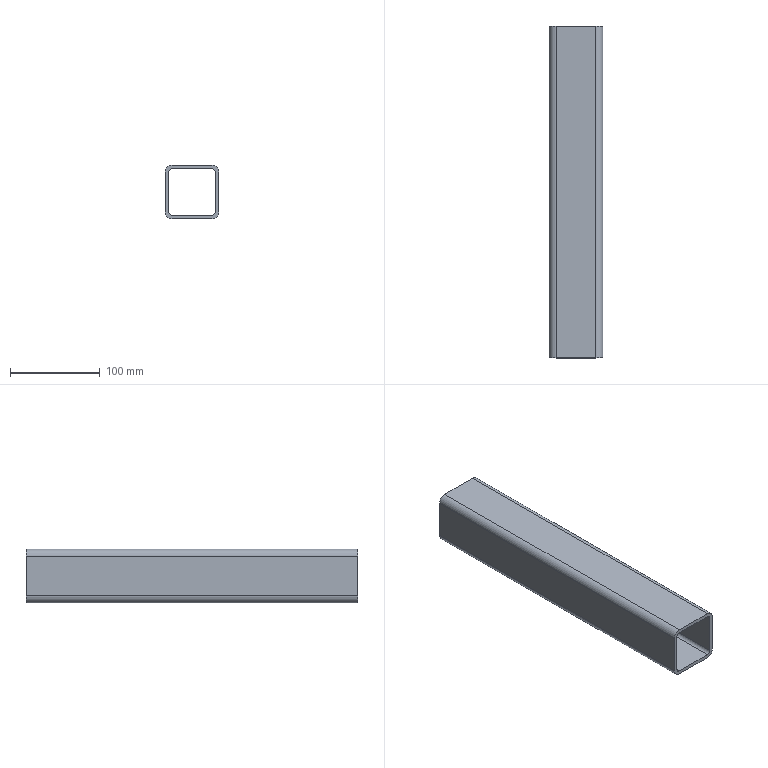Part | SolidWorks | features BaseBody 1 | 1 solid | 18 faces | box 60 x 370 x 60 mm | volume 316275 mm3 | plane 10 | cylinder 8 | commonest cylinder face diameters 8 x4 16 x4
STEP:
#1=CARTESIAN_POINT('',(26.,2432.,-1308.));
#2=VERTEX_POINT('',#1);
#3=CARTESIAN_POINT('',(26.,2432.,-1352.));
#4=VERTEX_POINT('',#3);
#5=CARTESIAN_POINT('',(26.,2432.,-1308.));
#6=DIRECTION('',(0.,0.,-1.));
#7=VECTOR('',#6,1000.);
#8=LINE('',#5,#7);
#9=EDGE_CURVE('',#2,#4,#8,.T.);
#10=ORIENTED_EDGE('',*,*,#9,.T.);
#11=CARTESIAN_POINT('',(26.,2062.,-1352.));
#12=VERTEX_POINT('',#11);
#13=CARTESIAN_POINT('',(26.,2432.,-1352.));
#14=DIRECTION('',(0.,-1.,0.));
#15=VECTOR('',#14,1000.);
#16=LINE('',#13,#15);
#17=EDGE_CURVE('',#4,#12,#16,.T.);
#18=ORIENTED_EDGE('',*,*,#17,.T.);
#19=CARTESIAN_POINT('',(26.,2062.,-1308.));
#20=VERTEX_POINT('',#19);
#21=CARTESIAN_POINT('',(26.,2062.,-1308.));
#22=DIRECTION('',(0.,0.,1.));
#23=VECTOR('',#22,1000.);
#24=LINE('',#21,#23);
#25=EDGE_CURVE('',#12,#20,#24,.T.);
#26=ORIENTED_EDGE('',*,*,#25,.T.);
#27=CARTESIAN_POINT('',(26.,2432.,-1308.));
#28=DIRECTION('',(0.,1.,0.));
#29=VECTOR('',#28,1000.);
#30=LINE('',#27,#29);
#31=EDGE_CURVE('',#20,#2,#30,.T.);
#32=ORIENTED_EDGE('',*,*,#31,.T.);
#33=EDGE_LOOP('',(#10,#18,#26,#32));
#34=FACE_OUTER_BOUND('',#33,.T.);
#35=CARTESIAN_POINT('',(26.,2432.,-1308.));
#36=DIRECTION('',(-1.,0.,0.));
#37=DIRECTION('',(0.,0.,1.));
#38=AXIS2_PLACEMENT_3D('',#35,#36,#37);
#39=PLANE('',#38);
#40=ADVANCED_FACE('',(#34),#39,.T.);
#41=ORIENTED_EDGE('',*,*,#17,.F.);
#42=CARTESIAN_POINT('',(22.,2432.,-1356.));
#43=VERTEX_POINT('',#42);
#44=CARTESIAN_POINT('',(22.,2432.,-1352.));
#45=DIRECTION('',(0.,-1.,0.));
#46=DIRECTION('',(0.,0.,-1.));
#47=AXIS2_PLACEMENT_3D('',#44,#45,#46);
#48=CIRCLE('',#47,4.);
#49=EDGE_CURVE('',#43,#4,#48,.T.);
#50=ORIENTED_EDGE('',*,*,#49,.F.);
#51=CARTESIAN_POINT('',(22.,2062.,-1356.));
#52=VERTEX_POINT('',#51);
#53=CARTESIAN_POINT('',(22.,2432.,-1356.));
#54=DIRECTION('',(0.,1.,0.));
#55=VECTOR('',#54,1000.);
#56=LINE('',#53,#55);
#57=EDGE_CURVE('',#52,#43,#56,.T.);
#58=ORIENTED_EDGE('',*,*,#57,.F.);
#59=CARTESIAN_POINT('',(22.,2062.,-1352.));
#60=DIRECTION('',(0.,1.,0.));
#61=DIRECTION('',(0.,0.,-1.));
#62=AXIS2_PLACEMENT_3D('',#59,#60,#61);
#63=CIRCLE('',#62,4.);
#64=EDGE_CURVE('',#12,#52,#63,.T.);
#65=ORIENTED_EDGE('',*,*,#64,.F.);
#66=EDGE_LOOP('',(#41,#50,#58,#65));
#67=FACE_OUTER_BOUND('',#66,.T.);
#68=CARTESIAN_POINT('',(22.,2432.,-1352.));
#69=DIRECTION('',(0.,-1.,0.));
#70=DIRECTION('',(0.,0.,-1.));
#71=AXIS2_PLACEMENT_3D('',#68,#69,#70);
#72=CYLINDRICAL_SURFACE('',#71,4.);
#73=ADVANCED_FACE('',(#67),#72,.F.);
#74=CARTESIAN_POINT('',(22.,2432.,-1304.));
#75=VERTEX_POINT('',#74);
#76=CARTESIAN_POINT('',(-22.,2432.,-1304.));
#77=VERTEX_POINT('',#76);
#78=CARTESIAN_POINT('',(-22.,2432.,-1304.));
#79=DIRECTION('',(-1.,0.,0.));
#80=VECTOR('',#79,1000.);
#81=LINE('',#78,#80);
#82=EDGE_CURVE('',#75,#77,#81,.T.);
#83=ORIENTED_EDGE('',*,*,#82,.T.);
#84=CARTESIAN_POINT('',(-26.,2432.,-1308.));
#85=VERTEX_POINT('',#84);
#86=CARTESIAN_POINT('',(-22.,2432.,-1308.));
#87=DIRECTION('',(0.,-1.,0.));
#88=DIRECTION('',(0.,0.,-1.));
#89=AXIS2_PLACEMENT_3D('',#86,#87,#88);
#90=CIRCLE('',#89,4.);
#91=EDGE_CURVE('',#77,#85,#90,.T.);
#92=ORIENTED_EDGE('',*,*,#91,.T.);
#93=CARTESIAN_POINT('',(-26.,2432.,-1352.));
#94=VERTEX_POINT('',#93);
#95=CARTESIAN_POINT('',(-26.,2432.,-1352.));
#96=DIRECTION('',(0.,0.,-1.));
#97=VECTOR('',#96,1000.);
#98=LINE('',#95,#97);
#99=EDGE_CURVE('',#85,#94,#98,.T.);
#100=ORIENTED_EDGE('',*,*,#99,.T.);
#101=CARTESIAN_POINT('',(-22.,2432.,-1356.));
#102=VERTEX_POINT('',#101);
#103=CARTESIAN_POINT('',(-22.,2432.,-1352.));
#104=DIRECTION('',(0.,-1.,0.));
#105=DIRECTION('',(0.,0.,-1.));
#106=AXIS2_PLACEMENT_3D('',#103,#104,#105);
#107=CIRCLE('',#106,4.);
#108=EDGE_CURVE('',#94,#102,#107,.T.);
#109=ORIENTED_EDGE('',*,*,#108,.T.);
#110=CARTESIAN_POINT('',(-22.,2432.,-1356.));
#111=DIRECTION('',(1.,0.,0.));
#112=VECTOR('',#111,1000.);
#113=LINE('',#110,#112);
#114=EDGE_CURVE('',#102,#43,#113,.T.);
#115=ORIENTED_EDGE('',*,*,#114,.T.);
#116=ORIENTED_EDGE('',*,*,#49,.T.);
#117=ORIENTED_EDGE('',*,*,#9,.F.);
#118=CARTESIAN_POINT('',(22.,2432.,-1308.));
#119=DIRECTION('',(0.,-1.,0.));
#120=DIRECTION('',(0.,0.,-1.));
#121=AXIS2_PLACEMENT_3D('',#118,#119,#120);
#122=CIRCLE('',#121,4.);
#123=EDGE_CURVE('',#2,#75,#122,.T.);
#124=ORIENTED_EDGE('',*,*,#123,.T.);
#125=EDGE_LOOP('',(#83,#92,#100,#109,#115,#116,#117,#124));
#126=FACE_BOUND('',#125,.T.);
#127=CARTESIAN_POINT('',(22.,2432.,-1360.));
#128=VERTEX_POINT('',#127);
#129=CARTESIAN_POINT('',(-22.,2432.,-1360.));
#130=VERTEX_POINT('',#129);
#131=CARTESIAN_POINT('',(-22.,2432.,-1360.));
#132=DIRECTION('',(-1.,0.,0.));
#133=VECTOR('',#132,1000.);
#134=LINE('',#131,#133);
#135=EDGE_CURVE('',#128,#130,#134,.T.);
#136=ORIENTED_EDGE('',*,*,#135,.T.);
#137=CARTESIAN_POINT('',(-30.,2432.,-1352.));
#138=VERTEX_POINT('',#137);
#139=CARTESIAN_POINT('',(-22.,2432.,-1352.));
#140=DIRECTION('',(0.,1.,0.));
#141=DIRECTION('',(0.,0.,-1.));
#142=AXIS2_PLACEMENT_3D('',#139,#140,#141);
#143=CIRCLE('',#142,8.);
#144=EDGE_CURVE('',#130,#138,#143,.T.);
#145=ORIENTED_EDGE('',*,*,#144,.T.);
#146=CARTESIAN_POINT('',(-30.,2432.,-1308.));
#147=VERTEX_POINT('',#146);
#148=CARTESIAN_POINT('',(-30.,2432.,-1352.));
#149=DIRECTION('',(0.,0.,1.));
#150=VECTOR('',#149,1000.);
#151=LINE('',#148,#150);
#152=EDGE_CURVE('',#138,#147,#151,.T.);
#153=ORIENTED_EDGE('',*,*,#152,.T.);
#154=CARTESIAN_POINT('',(-22.,2432.,-1300.));
#155=VERTEX_POINT('',#154);
#156=CARTESIAN_POINT('',(-22.,2432.,-1308.));
#157=DIRECTION('',(0.,1.,0.));
#158=DIRECTION('',(0.,0.,-1.));
#159=AXIS2_PLACEMENT_3D('',#156,#157,#158);
#160=CIRCLE('',#159,8.);
#161=EDGE_CURVE('',#147,#155,#160,.T.);
#162=ORIENTED_EDGE('',*,*,#161,.T.);
#163=CARTESIAN_POINT('',(22.,2432.,-1300.));
#164=VERTEX_POINT('',#163);
#165=CARTESIAN_POINT('',(-22.,2432.,-1300.));
#166=DIRECTION('',(1.,0.,0.));
#167=VECTOR('',#166,1000.);
#168=LINE('',#165,#167);
#169=EDGE_CURVE('',#155,#164,#168,.T.);
#170=ORIENTED_EDGE('',*,*,#169,.T.);
#171=CARTESIAN_POINT('',(30.,2432.,-1308.));
#172=VERTEX_POINT('',#171);
#173=CARTESIAN_POINT('',(22.,2432.,-1308.));
#174=DIRECTION('',(0.,1.,0.));
#175=DIRECTION('',(0.,0.,-1.));
#176=AXIS2_PLACEMENT_3D('',#173,#174,#175);
#177=CIRCLE('',#176,8.);
#178=EDGE_CURVE('',#164,#172,#177,.T.);
#179=ORIENTED_EDGE('',*,*,#178,.T.);
#180=CARTESIAN_POINT('',(30.,2432.,-1352.));
#181=VERTEX_POINT('',#180);
#182=CARTESIAN_POINT('',(30.,2432.,-1352.));
#183=DIRECTION('',(0.,0.,-1.));
#184=VECTOR('',#183,1000.);
#185=LINE('',#182,#184);
#186=EDGE_CURVE('',#172,#181,#185,.T.);
#187=ORIENTED_EDGE('',*,*,#186,.T.);
#188=CARTESIAN_POINT('',(22.,2432.,-1352.));
#189=DIRECTION('',(0.,1.,0.));
#190=DIRECTION('',(0.,0.,-1.));
#191=AXIS2_PLACEMENT_3D('',#188,#189,#190);
#192=CIRCLE('',#191,8.);
#193=EDGE_CURVE('',#181,#128,#192,.T.);
#194=ORIENTED_EDGE('',*,*,#193,.T.);
#195=EDGE_LOOP('',(#136,#145,#153,#162,#170,#179,#187,#194));
#196=FACE_OUTER_BOUND('',#195,.T.);
#197=CARTESIAN_POINT('',(-22.,2432.,-1352.));
#198=DIRECTION('',(0.,1.,0.));
#199=DIRECTION('',(0.,0.,1.));
#200=AXIS2_PLACEMENT_3D('',#197,#198,#199);
#201=PLANE('',#200);
#202=ADVANCED_FACE('',(#126,#196),#201,.T.);
#203=CARTESIAN_POINT('',(22.,2062.,-1304.));
#204=VERTEX_POINT('',#203);
#205=CARTESIAN_POINT('',(22.,2432.,-1304.));
#206=DIRECTION('',(0.,-1.,0.));
#207=VECTOR('',#206,1000.);
#208=LINE('',#205,#207);
#209=EDGE_CURVE('',#75,#204,#208,.T.);
#210=ORIENTED_EDGE('',*,*,#209,.F.);
#211=ORIENTED_EDGE('',*,*,#123,.F.);
#212=ORIENTED_EDGE('',*,*,#31,.F.);
#213=CARTESIAN_POINT('',(22.,2062.,-1308.));
#214=DIRECTION('',(0.,1.,0.));
#215=DIRECTION('',(0.,0.,-1.));
#216=AXIS2_PLACEMENT_3D('',#213,#214,#215);
#217=CIRCLE('',#216,4.);
#218=EDGE_CURVE('',#204,#20,#217,.T.);
#219=ORIENTED_EDGE('',*,*,#218,.F.);
#220=EDGE_LOOP('',(#210,#211,#212,#219));
#221=FACE_OUTER_BOUND('',#220,.T.);
#222=CARTESIAN_POINT('',(22.,2432.,-1308.));
#223=DIRECTION('',(0.,-1.,0.));
#224=DIRECTION('',(0.,0.,-1.));
#225=AXIS2_PLACEMENT_3D('',#222,#223,#224);
#226=CYLINDRICAL_SURFACE('',#225,4.);
#227=ADVANCED_FACE('',(#221),#226,.F.);
#228=CARTESIAN_POINT('',(-26.,2062.,-1308.));
#229=VERTEX_POINT('',#228);
#230=CARTESIAN_POINT('',(-22.,2062.,-1304.));
#231=VERTEX_POINT('',#230);
#232=CARTESIAN_POINT('',(-22.,2062.,-1308.));
#233=DIRECTION('',(0.,1.,0.));
#234=DIRECTION('',(0.,0.,-1.));
#235=AXIS2_PLACEMENT_3D('',#232,#233,#234);
#236=CIRCLE('',#235,4.);
#237=EDGE_CURVE('',#229,#231,#236,.T.);
#238=ORIENTED_EDGE('',*,*,#237,.T.);
#239=CARTESIAN_POINT('',(-22.,2062.,-1304.));
#240=DIRECTION('',(1.,0.,0.));
#241=VECTOR('',#240,1000.);
#242=LINE('',#239,#241);
#243=EDGE_CURVE('',#231,#204,#242,.T.);
#244=ORIENTED_EDGE('',*,*,#243,.T.);
#245=ORIENTED_EDGE('',*,*,#218,.T.);
#246=ORIENTED_EDGE('',*,*,#25,.F.);
#247=ORIENTED_EDGE('',*,*,#64,.T.);
#248=CARTESIAN_POINT('',(-22.,2062.,-1356.));
#249=VERTEX_POINT('',#248);
#250=CARTESIAN_POINT('',(-22.,2062.,-1356.));
#251=DIRECTION('',(-1.,0.,0.));
#252=VECTOR('',#251,1000.);
#253=LINE('',#250,#252);
#254=EDGE_CURVE('',#52,#249,#253,.T.);
#255=ORIENTED_EDGE('',*,*,#254,.T.);
#256=CARTESIAN_POINT('',(-26.,2062.,-1352.));
#257=VERTEX_POINT('',#256);
#258=CARTESIAN_POINT('',(-22.,2062.,-1352.));
#259=DIRECTION('',(0.,1.,0.));
#260=DIRECTION('',(0.,0.,-1.));
#261=AXIS2_PLACEMENT_3D('',#258,#259,#260);
#262=CIRCLE('',#261,4.);
#263=EDGE_CURVE('',#249,#257,#262,.T.);
#264=ORIENTED_EDGE('',*,*,#263,.T.);
#265=CARTESIAN_POINT('',(-26.,2062.,170.));
#266=DIRECTION('',(0.,0.,1.));
#267=VECTOR('',#266,1000.);
#268=LINE('',#265,#267);
#269=EDGE_CURVE('',#257,#229,#268,.T.);
#270=ORIENTED_EDGE('',*,*,#269,.T.);
#271=EDGE_LOOP('',(#238,#244,#245,#246,#247,#255,#264,#270));
#272=FACE_BOUND('',#271,.T.);
#273=CARTESIAN_POINT('',(22.,2062.,-1300.));
#274=VERTEX_POINT('',#273);
#275=CARTESIAN_POINT('',(-22.,2062.,-1300.));
#276=VERTEX_POINT('',#275);
#277=CARTESIAN_POINT('',(-22.,2062.,-1300.));
#278=DIRECTION('',(-1.,0.,0.));
#279=VECTOR('',#278,1000.);
#280=LINE('',#277,#279);
#281=EDGE_CURVE('',#274,#276,#280,.T.);
#282=ORIENTED_EDGE('',*,*,#281,.T.);
#283=CARTESIAN_POINT('',(-30.,2062.,-1308.));
#284=VERTEX_POINT('',#283);
#285=CARTESIAN_POINT('',(-22.,2062.,-1308.));
#286=DIRECTION('',(0.,-1.,0.));
#287=DIRECTION('',(0.,0.,-1.));
#288=AXIS2_PLACEMENT_3D('',#285,#286,#287);
#289=CIRCLE('',#288,8.);
#290=EDGE_CURVE('',#276,#284,#289,.T.);
#291=ORIENTED_EDGE('',*,*,#290,.T.);
#292=CARTESIAN_POINT('',(-30.,2062.,-1352.));
#293=VERTEX_POINT('',#292);
#294=CARTESIAN_POINT('',(-30.,2062.,170.));
#295=DIRECTION('',(0.,0.,-1.));
#296=VECTOR('',#295,1000.);
#297=LINE('',#294,#296);
#298=EDGE_CURVE('',#284,#293,#297,.T.);
#299=ORIENTED_EDGE('',*,*,#298,.T.);
#300=CARTESIAN_POINT('',(-22.,2062.,-1360.));
#301=VERTEX_POINT('',#300);
#302=CARTESIAN_POINT('',(-22.,2062.,-1352.));
#303=DIRECTION('',(0.,-1.,0.));
#304=DIRECTION('',(0.,0.,-1.));
#305=AXIS2_PLACEMENT_3D('',#302,#303,#304);
#306=CIRCLE('',#305,8.);
#307=EDGE_CURVE('',#293,#301,#306,.T.);
#308=ORIENTED_EDGE('',*,*,#307,.T.);
#309=CARTESIAN_POINT('',(22.,2062.,-1360.));
#310=VERTEX_POINT('',#309);
#311=CARTESIAN_POINT('',(-22.,2062.,-1360.));
#312=DIRECTION('',(1.,0.,0.));
#313=VECTOR('',#312,1000.);
#314=LINE('',#311,#313);
#315=EDGE_CURVE('',#301,#310,#314,.T.);
#316=ORIENTED_EDGE('',*,*,#315,.T.);
#317=CARTESIAN_POINT('',(30.,2062.,-1352.));
#318=VERTEX_POINT('',#317);
#319=CARTESIAN_POINT('',(22.,2062.,-1352.));
#320=DIRECTION('',(0.,-1.,0.));
#321=DIRECTION('',(0.,0.,-1.));
#322=AXIS2_PLACEMENT_3D('',#319,#320,#321);
#323=CIRCLE('',#322,8.);
#324=EDGE_CURVE('',#310,#318,#323,.T.);
#325=ORIENTED_EDGE('',*,*,#324,.T.);
#326=CARTESIAN_POINT('',(30.,2062.,-1308.));
#327=VERTEX_POINT('',#326);
#328=CARTESIAN_POINT('',(30.,2062.,170.));
#329=DIRECTION('',(0.,0.,1.));
#330=VECTOR('',#329,1000.);
#331=LINE('',#328,#330);
#332=EDGE_CURVE('',#318,#327,#331,.T.);
#333=ORIENTED_EDGE('',*,*,#332,.T.);
#334=CARTESIAN_POINT('',(22.,2062.,-1308.));
#335=DIRECTION('',(0.,-1.,0.));
#336=DIRECTION('',(0.,0.,-1.));
#337=AXIS2_PLACEMENT_3D('',#334,#335,#336);
#338=CIRCLE('',#337,8.);
#339=EDGE_CURVE('',#327,#274,#338,.T.);
#340=ORIENTED_EDGE('',*,*,#339,.T.);
#341=EDGE_LOOP('',(#282,#291,#299,#308,#316,#325,#333,#340));
#342=FACE_OUTER_BOUND('',#341,.T.);
#343=CARTESIAN_POINT('',(-22.,2062.,170.));
#344=DIRECTION('',(0.,-1.,0.));
#345=DIRECTION('',(0.,0.,-1.));
#346=AXIS2_PLACEMENT_3D('',#343,#344,#345);
#347=PLANE('',#346);
#348=ADVANCED_FACE('',(#272,#342),#347,.T.);
#349=ORIENTED_EDGE('',*,*,#114,.F.);
#350=CARTESIAN_POINT('',(-22.,2432.,-1356.));
#351=DIRECTION('',(0.,-1.,0.));
#352=VECTOR('',#351,1000.);
#353=LINE('',#350,#352);
#354=EDGE_CURVE('',#102,#249,#353,.T.);
#355=ORIENTED_EDGE('',*,*,#354,.T.);
#356=ORIENTED_EDGE('',*,*,#254,.F.);
#357=ORIENTED_EDGE('',*,*,#57,.T.);
#358=EDGE_LOOP('',(#349,#355,#356,#357));
#359=FACE_OUTER_BOUND('',#358,.T.);
#360=CARTESIAN_POINT('',(-22.,2432.,-1356.));
#361=DIRECTION('',(0.,0.,1.));
#362=DIRECTION('',(1.,0.,0.));
#363=AXIS2_PLACEMENT_3D('',#360,#361,#362);
#364=PLANE('',#363);
#365=ADVANCED_FACE('',(#359),#364,.T.);
#366=CARTESIAN_POINT('',(-26.,2432.,-1308.));
#367=DIRECTION('',(0.,-1.,0.));
#368=VECTOR('',#367,1000.);
#369=LINE('',#366,#368);
#370=EDGE_CURVE('',#85,#229,#369,.T.);
#371=ORIENTED_EDGE('',*,*,#370,.F.);
#372=ORIENTED_EDGE('',*,*,#91,.F.);
#373=CARTESIAN_POINT('',(-22.,2432.,-1304.));
#374=DIRECTION('',(0.,1.,0.));
#375=VECTOR('',#374,1000.);
#376=LINE('',#373,#375);
#377=EDGE_CURVE('',#231,#77,#376,.T.);
#378=ORIENTED_EDGE('',*,*,#377,.F.);
#379=ORIENTED_EDGE('',*,*,#237,.F.);
#380=EDGE_LOOP('',(#371,#372,#378,#379));
#381=FACE_OUTER_BOUND('',#380,.T.);
#382=CARTESIAN_POINT('',(-22.,2432.,-1308.));
#383=DIRECTION('',(0.,-1.,0.));
#384=DIRECTION('',(0.,0.,-1.));
#385=AXIS2_PLACEMENT_3D('',#382,#383,#384);
#386=CYLINDRICAL_SURFACE('',#385,4.);
#387=ADVANCED_FACE('',(#381),#386,.F.);
#388=ORIENTED_EDGE('',*,*,#82,.F.);
#389=ORIENTED_EDGE('',*,*,#209,.T.);
#390=ORIENTED_EDGE('',*,*,#243,.F.);
#391=ORIENTED_EDGE('',*,*,#377,.T.);
#392=EDGE_LOOP('',(#388,#389,#390,#391));
#393=FACE_OUTER_BOUND('',#392,.T.);
#394=CARTESIAN_POINT('',(22.,2432.,-1304.));
#395=DIRECTION('',(0.,0.,-1.));
#396=DIRECTION('',(-1.,0.,0.));
#397=AXIS2_PLACEMENT_3D('',#394,#395,#396);
#398=PLANE('',#397);
#399=ADVANCED_FACE('',(#393),#398,.T.);
#400=ORIENTED_EDGE('',*,*,#354,.F.);
#401=ORIENTED_EDGE('',*,*,#108,.F.);
#402=CARTESIAN_POINT('',(-26.,2432.,-1352.));
#403=DIRECTION('',(0.,1.,0.));
#404=VECTOR('',#403,1000.);
#405=LINE('',#402,#404);
#406=EDGE_CURVE('',#257,#94,#405,.T.);
#407=ORIENTED_EDGE('',*,*,#406,.F.);
#408=ORIENTED_EDGE('',*,*,#263,.F.);
#409=EDGE_LOOP('',(#400,#401,#407,#408));
#410=FACE_OUTER_BOUND('',#409,.T.);
#411=CARTESIAN_POINT('',(-22.,2432.,-1352.));
#412=DIRECTION('',(0.,-1.,0.));
#413=DIRECTION('',(0.,0.,-1.));
#414=AXIS2_PLACEMENT_3D('',#411,#412,#413);
#415=CYLINDRICAL_SURFACE('',#414,4.);
#416=ADVANCED_FACE('',(#410),#415,.F.);
#417=ORIENTED_EDGE('',*,*,#99,.F.);
#418=ORIENTED_EDGE('',*,*,#370,.T.);
#419=ORIENTED_EDGE('',*,*,#269,.F.);
#420=ORIENTED_EDGE('',*,*,#406,.T.);
#421=EDGE_LOOP('',(#417,#418,#419,#420));
#422=FACE_OUTER_BOUND('',#421,.T.);
#423=CARTESIAN_POINT('',(-26.,2432.,-1352.));
#424=DIRECTION('',(1.,0.,0.));
#425=DIRECTION('',(0.,0.,-1.));
#426=AXIS2_PLACEMENT_3D('',#423,#424,#425);
#427=PLANE('',#426);
#428=ADVANCED_FACE('',(#422),#427,.T.);
#429=CARTESIAN_POINT('',(-22.,2432.,-1360.));
#430=DIRECTION('',(0.,-1.,0.));
#431=VECTOR('',#430,1000.);
#432=LINE('',#429,#431);
#433=EDGE_CURVE('',#130,#301,#432,.T.);
#434=ORIENTED_EDGE('',*,*,#433,.T.);
#435=ORIENTED_EDGE('',*,*,#307,.F.);
#436=CARTESIAN_POINT('',(-30.,2432.,-1352.));
#437=DIRECTION('',(0.,1.,0.));
#438=VECTOR('',#437,1000.);
#439=LINE('',#436,#438);
#440=EDGE_CURVE('',#293,#138,#439,.T.);
#441=ORIENTED_EDGE('',*,*,#440,.T.);
#442=ORIENTED_EDGE('',*,*,#144,.F.);
#443=EDGE_LOOP('',(#434,#435,#441,#442));
#444=FACE_OUTER_BOUND('',#443,.T.);
#445=CARTESIAN_POINT('',(-22.,2432.,-1352.));
#446=DIRECTION('',(0.,-1.,0.));
#447=DIRECTION('',(0.,0.,-1.));
#448=AXIS2_PLACEMENT_3D('',#445,#446,#447);
#449=CYLINDRICAL_SURFACE('',#448,8.);
#450=ADVANCED_FACE('',(#444),#449,.T.);
#451=ORIENTED_EDGE('',*,*,#135,.F.);
#452=CARTESIAN_POINT('',(22.,2432.,-1360.));
#453=DIRECTION('',(0.,1.,0.));
#454=VECTOR('',#453,1000.);
#455=LINE('',#452,#454);
#456=EDGE_CURVE('',#310,#128,#455,.T.);
#457=ORIENTED_EDGE('',*,*,#456,.F.);
#458=ORIENTED_EDGE('',*,*,#315,.F.);
#459=ORIENTED_EDGE('',*,*,#433,.F.);
#460=EDGE_LOOP('',(#451,#457,#458,#459));
#461=FACE_OUTER_BOUND('',#460,.T.);
#462=CARTESIAN_POINT('',(-22.,2432.,-1360.));
#463=DIRECTION('',(0.,0.,1.));
#464=DIRECTION('',(1.,0.,0.));
#465=AXIS2_PLACEMENT_3D('',#462,#463,#464);
#466=PLANE('',#465);
#467=ADVANCED_FACE('',(#461),#466,.F.);
#468=CARTESIAN_POINT('',(30.,2432.,-1352.));
#469=DIRECTION('',(0.,-1.,0.));
#470=VECTOR('',#469,1000.);
#471=LINE('',#468,#470);
#472=EDGE_CURVE('',#181,#318,#471,.T.);
#473=ORIENTED_EDGE('',*,*,#472,.T.);
#474=ORIENTED_EDGE('',*,*,#324,.F.);
#475=ORIENTED_EDGE('',*,*,#456,.T.);
#476=ORIENTED_EDGE('',*,*,#193,.F.);
#477=EDGE_LOOP('',(#473,#474,#475,#476));
#478=FACE_OUTER_BOUND('',#477,.T.);
#479=CARTESIAN_POINT('',(22.,2432.,-1352.));
#480=DIRECTION('',(0.,-1.,0.));
#481=DIRECTION('',(0.,0.,-1.));
#482=AXIS2_PLACEMENT_3D('',#479,#480,#481);
#483=CYLINDRICAL_SURFACE('',#482,8.);
#484=ADVANCED_FACE('',(#478),#483,.T.);
#485=ORIENTED_EDGE('',*,*,#186,.F.);
#486=CARTESIAN_POINT('',(30.,2432.,-1308.));
#487=DIRECTION('',(0.,1.,0.));
#488=VECTOR('',#487,1000.);
#489=LINE('',#486,#488);
#490=EDGE_CURVE('',#327,#172,#489,.T.);
#491=ORIENTED_EDGE('',*,*,#490,.F.);
#492=ORIENTED_EDGE('',*,*,#332,.F.);
#493=ORIENTED_EDGE('',*,*,#472,.F.);
#494=EDGE_LOOP('',(#485,#491,#492,#493));
#495=FACE_OUTER_BOUND('',#494,.T.);
#496=CARTESIAN_POINT('',(30.,2432.,-1308.));
#497=DIRECTION('',(-1.,0.,0.));
#498=DIRECTION('',(0.,0.,1.));
#499=AXIS2_PLACEMENT_3D('',#496,#497,#498);
#500=PLANE('',#499);
#501=ADVANCED_FACE('',(#495),#500,.F.);
#502=CARTESIAN_POINT('',(22.,2432.,-1300.));
#503=DIRECTION('',(0.,-1.,0.));
#504=VECTOR('',#503,1000.);
#505=LINE('',#502,#504);
#506=EDGE_CURVE('',#164,#274,#505,.T.);
#507=ORIENTED_EDGE('',*,*,#506,.T.);
#508=ORIENTED_EDGE('',*,*,#339,.F.);
#509=ORIENTED_EDGE('',*,*,#490,.T.);
#510=ORIENTED_EDGE('',*,*,#178,.F.);
#511=EDGE_LOOP('',(#507,#508,#509,#510));
#512=FACE_OUTER_BOUND('',#511,.T.);
#513=CARTESIAN_POINT('',(22.,2432.,-1308.));
#514=DIRECTION('',(0.,-1.,0.));
#515=DIRECTION('',(0.,0.,-1.));
#516=AXIS2_PLACEMENT_3D('',#513,#514,#515);
#517=CYLINDRICAL_SURFACE('',#516,8.);
#518=ADVANCED_FACE('',(#512),#517,.T.);
#519=ORIENTED_EDGE('',*,*,#169,.F.);
#520=CARTESIAN_POINT('',(-22.,2432.,-1300.));
#521=DIRECTION('',(0.,1.,0.));
#522=VECTOR('',#521,1000.);
#523=LINE('',#520,#522);
#524=EDGE_CURVE('',#276,#155,#523,.T.);
#525=ORIENTED_EDGE('',*,*,#524,.F.);
#526=ORIENTED_EDGE('',*,*,#281,.F.);
#527=ORIENTED_EDGE('',*,*,#506,.F.);
#528=EDGE_LOOP('',(#519,#525,#526,#527));
#529=FACE_OUTER_BOUND('',#528,.T.);
#530=CARTESIAN_POINT('',(22.,2432.,-1300.));
#531=DIRECTION('',(0.,0.,-1.));
#532=DIRECTION('',(-1.,0.,0.));
#533=AXIS2_PLACEMENT_3D('',#530,#531,#532);
#534=PLANE('',#533);
#535=ADVANCED_FACE('',(#529),#534,.F.);
#536=CARTESIAN_POINT('',(-30.,2432.,-1308.));
#537=DIRECTION('',(0.,-1.,0.));
#538=VECTOR('',#537,1000.);
#539=LINE('',#536,#538);
#540=EDGE_CURVE('',#147,#284,#539,.T.);
#541=ORIENTED_EDGE('',*,*,#540,.T.);
#542=ORIENTED_EDGE('',*,*,#290,.F.);
#543=ORIENTED_EDGE('',*,*,#524,.T.);
#544=ORIENTED_EDGE('',*,*,#161,.F.);
#545=EDGE_LOOP('',(#541,#542,#543,#544));
#546=FACE_OUTER_BOUND('',#545,.T.);
#547=CARTESIAN_POINT('',(-22.,2432.,-1308.));
#548=DIRECTION('',(0.,-1.,0.));
#549=DIRECTION('',(0.,0.,-1.));
#550=AXIS2_PLACEMENT_3D('',#547,#548,#549);
#551=CYLINDRICAL_SURFACE('',#550,8.);
#552=ADVANCED_FACE('',(#546),#551,.T.);
#553=ORIENTED_EDGE('',*,*,#152,.F.);
#554=ORIENTED_EDGE('',*,*,#440,.F.);
#555=ORIENTED_EDGE('',*,*,#298,.F.);
#556=ORIENTED_EDGE('',*,*,#540,.F.);
#557=EDGE_LOOP('',(#553,#554,#555,#556));
#558=FACE_OUTER_BOUND('',#557,.T.);
#559=CARTESIAN_POINT('',(-30.,2432.,-1352.));
#560=DIRECTION('',(1.,0.,0.));
#561=DIRECTION('',(0.,0.,-1.));
#562=AXIS2_PLACEMENT_3D('',#559,#560,#561);
#563=PLANE('',#562);
#564=ADVANCED_FACE('',(#558),#563,.F.);
#565=CLOSED_SHELL('',(#40,#73,#202,#227,#348,#365,#387,#399,#416,#428,#450,#467,#484,#501,#518,#535,#552,#564));
#566=MANIFOLD_SOLID_BREP('',#565);
#567=CARTESIAN_POINT('',(0.,0.,0.));
#568=DIRECTION('',(0.,0.,1.));
#569=DIRECTION('',(1.,0.,0.));
#570=AXIS2_PLACEMENT_3D('',#567,#568,#569);
#571=(LENGTH_UNIT()NAMED_UNIT(*)SI_UNIT(.MILLI.,.METRE.));
#572=UNCERTAINTY_MEASURE_WITH_UNIT(LENGTH_MEASURE(0.00001),#571,'','');
#573=(NAMED_UNIT(*)PLANE_ANGLE_UNIT()SI_UNIT($,.RADIAN.));
#574=(NAMED_UNIT(*)SI_UNIT($,.STERADIAN.)SOLID_ANGLE_UNIT());
#575=(GEOMETRIC_REPRESENTATION_CONTEXT(3)GLOBAL_UNCERTAINTY_ASSIGNED_CONTEXT((#572))GLOBAL_UNIT_ASSIGNED_CONTEXT((#571,#573,#574))REPRESENTATION_CONTEXT('',''));
#576=ADVANCED_BREP_SHAPE_REPRESENTATION('',(#566,#570),#575);